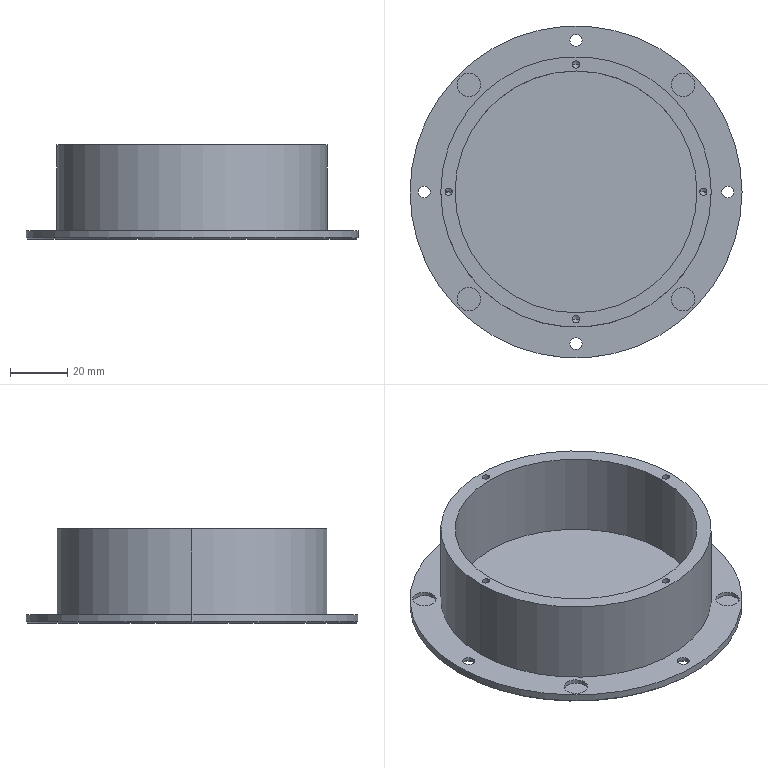Part | SolidWorks | features HoleWzd 2, ICE 2, Chamfer 1, Extrusion 1 | 1 solid | 56 faces | box 116 x 116 x 33 mm | volume 73097 mm3 | cylinder 30 | cone 18 | plane 8 | commonest cylinder face diameters 2.5 x8 4.2 x8 8.2 x8 84.5 x2 94.5 x2 116 x2
STEP:
#1=CARTESIAN_POINT('',(-41.577,-37.477,1.6));
#2=VERTEX_POINT('',#1);
#3=CARTESIAN_POINT('',(-33.377,-37.477,1.6));
#4=VERTEX_POINT('',#3);
#5=CARTESIAN_POINT('',(-37.477,-37.477,1.6));
#6=DIRECTION('',(0.,0.,1.));
#7=DIRECTION('',(-1.,0.,0.));
#8=AXIS2_PLACEMENT_3D('',#5,#6,#7);
#9=CIRCLE('',#8,4.1);
#10=EDGE_CURVE('',#2,#4,#9,.T.);
#11=ORIENTED_EDGE('',*,*,#10,.F.);
#12=CARTESIAN_POINT('',(-41.577,-37.477,3.));
#13=VERTEX_POINT('',#12);
#14=CARTESIAN_POINT('',(-41.577,-37.477,1.6));
#15=DIRECTION('',(0.,0.,1.));
#16=VECTOR('',#15,1000.);
#17=LINE('',#14,#16);
#18=EDGE_CURVE('',#2,#13,#17,.T.);
#19=ORIENTED_EDGE('',*,*,#18,.T.);
#20=CARTESIAN_POINT('',(-33.377,-37.477,3.));
#21=VERTEX_POINT('',#20);
#22=CARTESIAN_POINT('',(-37.477,-37.477,3.));
#23=DIRECTION('',(0.,0.,1.));
#24=DIRECTION('',(-1.,0.,0.));
#25=AXIS2_PLACEMENT_3D('',#22,#23,#24);
#26=CIRCLE('',#25,4.1);
#27=EDGE_CURVE('',#13,#21,#26,.T.);
#28=ORIENTED_EDGE('',*,*,#27,.T.);
#29=CARTESIAN_POINT('',(-33.377,-37.477,1.6));
#30=DIRECTION('',(0.,0.,1.));
#31=VECTOR('',#30,1000.);
#32=LINE('',#29,#31);
#33=EDGE_CURVE('',#4,#21,#32,.T.);
#34=ORIENTED_EDGE('',*,*,#33,.F.);
#35=EDGE_LOOP('',(#11,#19,#28,#34));
#36=FACE_OUTER_BOUND('',#35,.T.);
#37=CARTESIAN_POINT('',(-37.477,-37.477,1.6));
#38=DIRECTION('',(0.,0.,1.));
#39=DIRECTION('',(1.,0.,0.));
#40=AXIS2_PLACEMENT_3D('',#37,#38,#39);
#41=CYLINDRICAL_SURFACE('',#40,4.1);
#42=ADVANCED_FACE('',(#36),#41,.F.);
#43=CARTESIAN_POINT('',(-41.577,37.477,1.6));
#44=VERTEX_POINT('',#43);
#45=CARTESIAN_POINT('',(-33.377,37.477,1.6));
#46=VERTEX_POINT('',#45);
#47=CARTESIAN_POINT('',(-37.477,37.477,1.6));
#48=DIRECTION('',(0.,0.,1.));
#49=DIRECTION('',(1.,0.,0.));
#50=AXIS2_PLACEMENT_3D('',#47,#48,#49);
#51=CIRCLE('',#50,4.1);
#52=EDGE_CURVE('',#44,#46,#51,.T.);
#53=ORIENTED_EDGE('',*,*,#52,.F.);
#54=CARTESIAN_POINT('',(-41.577,37.477,3.));
#55=VERTEX_POINT('',#54);
#56=CARTESIAN_POINT('',(-41.577,37.477,1.6));
#57=DIRECTION('',(0.,0.,1.));
#58=VECTOR('',#57,1000.);
#59=LINE('',#56,#58);
#60=EDGE_CURVE('',#44,#55,#59,.T.);
#61=ORIENTED_EDGE('',*,*,#60,.T.);
#62=CARTESIAN_POINT('',(-33.377,37.477,3.));
#63=VERTEX_POINT('',#62);
#64=CARTESIAN_POINT('',(-37.477,37.477,3.));
#65=DIRECTION('',(0.,0.,1.));
#66=DIRECTION('',(1.,0.,0.));
#67=AXIS2_PLACEMENT_3D('',#64,#65,#66);
#68=CIRCLE('',#67,4.1);
#69=EDGE_CURVE('',#55,#63,#68,.T.);
#70=ORIENTED_EDGE('',*,*,#69,.T.);
#71=CARTESIAN_POINT('',(-33.377,37.477,1.6));
#72=DIRECTION('',(0.,0.,1.));
#73=VECTOR('',#72,1000.);
#74=LINE('',#71,#73);
#75=EDGE_CURVE('',#46,#63,#74,.T.);
#76=ORIENTED_EDGE('',*,*,#75,.F.);
#77=EDGE_LOOP('',(#53,#61,#70,#76));
#78=FACE_OUTER_BOUND('',#77,.T.);
#79=CARTESIAN_POINT('',(-37.477,37.477,1.6));
#80=DIRECTION('',(0.,0.,1.));
#81=DIRECTION('',(1.,0.,0.));
#82=AXIS2_PLACEMENT_3D('',#79,#80,#81);
#83=CYLINDRICAL_SURFACE('',#82,4.1);
#84=ADVANCED_FACE('',(#78),#83,.F.);
#85=CARTESIAN_POINT('',(33.377,37.477,1.6));
#86=VERTEX_POINT('',#85);
#87=CARTESIAN_POINT('',(41.577,37.477,1.6));
#88=VERTEX_POINT('',#87);
#89=CARTESIAN_POINT('',(37.477,37.477,1.6));
#90=DIRECTION('',(0.,0.,1.));
#91=DIRECTION('',(-1.,0.,0.));
#92=AXIS2_PLACEMENT_3D('',#89,#90,#91);
#93=CIRCLE('',#92,4.1);
#94=EDGE_CURVE('',#86,#88,#93,.T.);
#95=ORIENTED_EDGE('',*,*,#94,.F.);
#96=CARTESIAN_POINT('',(33.377,37.477,3.));
#97=VERTEX_POINT('',#96);
#98=CARTESIAN_POINT('',(33.377,37.477,1.6));
#99=DIRECTION('',(0.,0.,1.));
#100=VECTOR('',#99,1000.);
#101=LINE('',#98,#100);
#102=EDGE_CURVE('',#86,#97,#101,.T.);
#103=ORIENTED_EDGE('',*,*,#102,.T.);
#104=CARTESIAN_POINT('',(41.577,37.477,3.));
#105=VERTEX_POINT('',#104);
#106=CARTESIAN_POINT('',(37.477,37.477,3.));
#107=DIRECTION('',(0.,0.,1.));
#108=DIRECTION('',(-1.,0.,0.));
#109=AXIS2_PLACEMENT_3D('',#106,#107,#108);
#110=CIRCLE('',#109,4.1);
#111=EDGE_CURVE('',#97,#105,#110,.T.);
#112=ORIENTED_EDGE('',*,*,#111,.T.);
#113=CARTESIAN_POINT('',(41.577,37.477,1.6));
#114=DIRECTION('',(0.,0.,1.));
#115=VECTOR('',#114,1000.);
#116=LINE('',#113,#115);
#117=EDGE_CURVE('',#88,#105,#116,.T.);
#118=ORIENTED_EDGE('',*,*,#117,.F.);
#119=EDGE_LOOP('',(#95,#103,#112,#118));
#120=FACE_OUTER_BOUND('',#119,.T.);
#121=CARTESIAN_POINT('',(37.477,37.477,1.6));
#122=DIRECTION('',(0.,0.,1.));
#123=DIRECTION('',(1.,0.,0.));
#124=AXIS2_PLACEMENT_3D('',#121,#122,#123);
#125=CYLINDRICAL_SURFACE('',#124,4.1);
#126=ADVANCED_FACE('',(#120),#125,.F.);
#127=CARTESIAN_POINT('',(33.377,-37.477,1.6));
#128=VERTEX_POINT('',#127);
#129=CARTESIAN_POINT('',(41.577,-37.477,1.6));
#130=VERTEX_POINT('',#129);
#131=CARTESIAN_POINT('',(37.477,-37.477,1.6));
#132=DIRECTION('',(0.,0.,1.));
#133=DIRECTION('',(1.,0.,0.));
#134=AXIS2_PLACEMENT_3D('',#131,#132,#133);
#135=CIRCLE('',#134,4.1);
#136=EDGE_CURVE('',#128,#130,#135,.T.);
#137=ORIENTED_EDGE('',*,*,#136,.F.);
#138=CARTESIAN_POINT('',(33.377,-37.477,3.));
#139=VERTEX_POINT('',#138);
#140=CARTESIAN_POINT('',(33.377,-37.477,1.6));
#141=DIRECTION('',(0.,0.,1.));
#142=VECTOR('',#141,1000.);
#143=LINE('',#140,#142);
#144=EDGE_CURVE('',#128,#139,#143,.T.);
#145=ORIENTED_EDGE('',*,*,#144,.T.);
#146=CARTESIAN_POINT('',(41.577,-37.477,3.));
#147=VERTEX_POINT('',#146);
#148=CARTESIAN_POINT('',(37.477,-37.477,3.));
#149=DIRECTION('',(0.,0.,1.));
#150=DIRECTION('',(1.,0.,0.));
#151=AXIS2_PLACEMENT_3D('',#148,#149,#150);
#152=CIRCLE('',#151,4.1);
#153=EDGE_CURVE('',#139,#147,#152,.T.);
#154=ORIENTED_EDGE('',*,*,#153,.T.);
#155=CARTESIAN_POINT('',(41.577,-37.477,1.6));
#156=DIRECTION('',(0.,0.,1.));
#157=VECTOR('',#156,1000.);
#158=LINE('',#155,#157);
#159=EDGE_CURVE('',#130,#147,#158,.T.);
#160=ORIENTED_EDGE('',*,*,#159,.F.);
#161=EDGE_LOOP('',(#137,#145,#154,#160));
#162=FACE_OUTER_BOUND('',#161,.T.);
#163=CARTESIAN_POINT('',(37.477,-37.477,1.6));
#164=DIRECTION('',(0.,0.,1.));
#165=DIRECTION('',(1.,0.,0.));
#166=AXIS2_PLACEMENT_3D('',#163,#164,#165);
#167=CYLINDRICAL_SURFACE('',#166,4.1);
#168=ADVANCED_FACE('',(#162),#167,.F.);
#169=CARTESIAN_POINT('',(-1.25,44.5,25.5));
#170=VERTEX_POINT('',#169);
#171=CARTESIAN_POINT('',(1.25,44.5,25.5));
#172=VERTEX_POINT('',#171);
#173=CARTESIAN_POINT('',(0.,44.5,25.5));
#174=DIRECTION('',(0.,0.,1.));
#175=DIRECTION('',(1.,0.,0.));
#176=AXIS2_PLACEMENT_3D('',#173,#174,#175);
#177=CIRCLE('',#176,1.25);
#178=EDGE_CURVE('',#170,#172,#177,.T.);
#179=ORIENTED_EDGE('',*,*,#178,.F.);
#180=CARTESIAN_POINT('',(-1.25,44.5,33.));
#181=VERTEX_POINT('',#180);
#182=CARTESIAN_POINT('',(-1.25,44.5,33.));
#183=DIRECTION('',(0.,0.,1.));
#184=VECTOR('',#183,1000.);
#185=LINE('',#182,#184);
#186=EDGE_CURVE('',#170,#181,#185,.T.);
#187=ORIENTED_EDGE('',*,*,#186,.T.);
#188=CARTESIAN_POINT('',(1.25,44.5,33.));
#189=VERTEX_POINT('',#188);
#190=CARTESIAN_POINT('',(0.,44.5,33.));
#191=DIRECTION('',(0.,0.,1.));
#192=DIRECTION('',(1.,0.,0.));
#193=AXIS2_PLACEMENT_3D('',#190,#191,#192);
#194=CIRCLE('',#193,1.25);
#195=EDGE_CURVE('',#181,#189,#194,.T.);
#196=ORIENTED_EDGE('',*,*,#195,.T.);
#197=CARTESIAN_POINT('',(1.25,44.5,33.));
#198=DIRECTION('',(0.,0.,1.));
#199=VECTOR('',#198,1000.);
#200=LINE('',#197,#199);
#201=EDGE_CURVE('',#172,#189,#200,.T.);
#202=ORIENTED_EDGE('',*,*,#201,.F.);
#203=EDGE_LOOP('',(#179,#187,#196,#202));
#204=FACE_OUTER_BOUND('',#203,.T.);
#205=CARTESIAN_POINT('',(0.,44.5,33.));
#206=DIRECTION('',(0.,0.,1.));
#207=DIRECTION('',(1.,0.,0.));
#208=AXIS2_PLACEMENT_3D('',#205,#206,#207);
#209=CYLINDRICAL_SURFACE('',#208,1.25);
#210=ADVANCED_FACE('',(#204),#209,.F.);
#211=CARTESIAN_POINT('',(0.,44.5,24.749));
#212=VERTEX_POINT('',#211);
#213=CARTESIAN_POINT('',(1.25,44.5,25.5));
#214=DIRECTION('',(0.8572,0.,0.515));
#215=VECTOR('',#214,1000.);
#216=LINE('',#213,#215);
#217=EDGE_CURVE('',#212,#172,#216,.T.);
#218=ORIENTED_EDGE('',*,*,#217,.F.);
#219=CARTESIAN_POINT('',(-1.25,44.5,25.5));
#220=DIRECTION('',(-0.8572,0.,0.515));
#221=VECTOR('',#220,1000.);
#222=LINE('',#219,#221);
#223=EDGE_CURVE('',#212,#170,#222,.T.);
#224=ORIENTED_EDGE('',*,*,#223,.T.);
#225=ORIENTED_EDGE('',*,*,#178,.T.);
#226=EDGE_LOOP('',(#218,#224,#225));
#227=FACE_OUTER_BOUND('',#226,.T.);
#228=CARTESIAN_POINT('',(0.,44.5,25.5));
#229=DIRECTION('',(0.,0.,1.));
#230=DIRECTION('',(1.,0.,0.));
#231=AXIS2_PLACEMENT_3D('',#228,#229,#230);
#232=CONICAL_SURFACE('',#231,1.25,1.03);
#233=ADVANCED_FACE('',(#227),#232,.F.);
#234=CARTESIAN_POINT('',(43.25,0.,25.5));
#235=VERTEX_POINT('',#234);
#236=CARTESIAN_POINT('',(45.75,0.,25.5));
#237=VERTEX_POINT('',#236);
#238=CARTESIAN_POINT('',(44.5,0.,25.5));
#239=DIRECTION('',(0.,0.,1.));
#240=DIRECTION('',(1.,0.,0.));
#241=AXIS2_PLACEMENT_3D('',#238,#239,#240);
#242=CIRCLE('',#241,1.25);
#243=EDGE_CURVE('',#235,#237,#242,.T.);
#244=ORIENTED_EDGE('',*,*,#243,.F.);
#245=CARTESIAN_POINT('',(43.25,0.,33.));
#246=VERTEX_POINT('',#245);
#247=CARTESIAN_POINT('',(43.25,0.,33.));
#248=DIRECTION('',(0.,0.,1.));
#249=VECTOR('',#248,1000.);
#250=LINE('',#247,#249);
#251=EDGE_CURVE('',#235,#246,#250,.T.);
#252=ORIENTED_EDGE('',*,*,#251,.T.);
#253=CARTESIAN_POINT('',(45.75,0.,33.));
#254=VERTEX_POINT('',#253);
#255=CARTESIAN_POINT('',(44.5,0.,33.));
#256=DIRECTION('',(0.,0.,1.));
#257=DIRECTION('',(1.,0.,0.));
#258=AXIS2_PLACEMENT_3D('',#255,#256,#257);
#259=CIRCLE('',#258,1.25);
#260=EDGE_CURVE('',#246,#254,#259,.T.);
#261=ORIENTED_EDGE('',*,*,#260,.T.);
#262=CARTESIAN_POINT('',(45.75,0.,33.));
#263=DIRECTION('',(0.,0.,1.));
#264=VECTOR('',#263,1000.);
#265=LINE('',#262,#264);
#266=EDGE_CURVE('',#237,#254,#265,.T.);
#267=ORIENTED_EDGE('',*,*,#266,.F.);
#268=EDGE_LOOP('',(#244,#252,#261,#267));
#269=FACE_OUTER_BOUND('',#268,.T.);
#270=CARTESIAN_POINT('',(44.5,0.,33.));
#271=DIRECTION('',(0.,0.,1.));
#272=DIRECTION('',(1.,0.,0.));
#273=AXIS2_PLACEMENT_3D('',#270,#271,#272);
#274=CYLINDRICAL_SURFACE('',#273,1.25);
#275=ADVANCED_FACE('',(#269),#274,.F.);
#276=CARTESIAN_POINT('',(44.5,0.,24.749));
#277=VERTEX_POINT('',#276);
#278=CARTESIAN_POINT('',(45.75,0.,25.5));
#279=DIRECTION('',(0.8572,0.,0.515));
#280=VECTOR('',#279,1000.);
#281=LINE('',#278,#280);
#282=EDGE_CURVE('',#277,#237,#281,.T.);
#283=ORIENTED_EDGE('',*,*,#282,.F.);
#284=CARTESIAN_POINT('',(43.25,0.,25.5));
#285=DIRECTION('',(-0.8572,0.,0.515));
#286=VECTOR('',#285,1000.);
#287=LINE('',#284,#286);
#288=EDGE_CURVE('',#277,#235,#287,.T.);
#289=ORIENTED_EDGE('',*,*,#288,.T.);
#290=ORIENTED_EDGE('',*,*,#243,.T.);
#291=EDGE_LOOP('',(#283,#289,#290));
#292=FACE_OUTER_BOUND('',#291,.T.);
#293=CARTESIAN_POINT('',(44.5,0.,25.5));
#294=DIRECTION('',(0.,0.,1.));
#295=DIRECTION('',(1.,0.,0.));
#296=AXIS2_PLACEMENT_3D('',#293,#294,#295);
#297=CONICAL_SURFACE('',#296,1.25,1.03);
#298=ADVANCED_FACE('',(#292),#297,.F.);
#299=CARTESIAN_POINT('',(-1.25,-44.5,25.5));
#300=VERTEX_POINT('',#299);
#301=CARTESIAN_POINT('',(1.25,-44.5,25.5));
#302=VERTEX_POINT('',#301);
#303=CARTESIAN_POINT('',(0.,-44.5,25.5));
#304=DIRECTION('',(0.,0.,1.));
#305=DIRECTION('',(1.,0.,0.));
#306=AXIS2_PLACEMENT_3D('',#303,#304,#305);
#307=CIRCLE('',#306,1.25);
#308=EDGE_CURVE('',#300,#302,#307,.T.);
#309=ORIENTED_EDGE('',*,*,#308,.F.);
#310=CARTESIAN_POINT('',(-1.25,-44.5,33.));
#311=VERTEX_POINT('',#310);
#312=CARTESIAN_POINT('',(-1.25,-44.5,33.));
#313=DIRECTION('',(0.,0.,1.));
#314=VECTOR('',#313,1000.);
#315=LINE('',#312,#314);
#316=EDGE_CURVE('',#300,#311,#315,.T.);
#317=ORIENTED_EDGE('',*,*,#316,.T.);
#318=CARTESIAN_POINT('',(1.25,-44.5,33.));
#319=VERTEX_POINT('',#318);
#320=CARTESIAN_POINT('',(0.,-44.5,33.));
#321=DIRECTION('',(0.,0.,1.));
#322=DIRECTION('',(1.,0.,0.));
#323=AXIS2_PLACEMENT_3D('',#320,#321,#322);
#324=CIRCLE('',#323,1.25);
#325=EDGE_CURVE('',#311,#319,#324,.T.);
#326=ORIENTED_EDGE('',*,*,#325,.T.);
#327=CARTESIAN_POINT('',(1.25,-44.5,33.));
#328=DIRECTION('',(0.,0.,1.));
#329=VECTOR('',#328,1000.);
#330=LINE('',#327,#329);
#331=EDGE_CURVE('',#302,#319,#330,.T.);
#332=ORIENTED_EDGE('',*,*,#331,.F.);
#333=EDGE_LOOP('',(#309,#317,#326,#332));
#334=FACE_OUTER_BOUND('',#333,.T.);
#335=CARTESIAN_POINT('',(0.,-44.5,33.));
#336=DIRECTION('',(0.,0.,1.));
#337=DIRECTION('',(1.,0.,0.));
#338=AXIS2_PLACEMENT_3D('',#335,#336,#337);
#339=CYLINDRICAL_SURFACE('',#338,1.25);
#340=ADVANCED_FACE('',(#334),#339,.F.);
#341=CARTESIAN_POINT('',(0.,-44.5,24.749));
#342=VERTEX_POINT('',#341);
#343=CARTESIAN_POINT('',(1.25,-44.5,25.5));
#344=DIRECTION('',(0.8572,0.,0.515));
#345=VECTOR('',#344,1000.);
#346=LINE('',#343,#345);
#347=EDGE_CURVE('',#342,#302,#346,.T.);
#348=ORIENTED_EDGE('',*,*,#347,.F.);
#349=CARTESIAN_POINT('',(-1.25,-44.5,25.5));
#350=DIRECTION('',(-0.8572,0.,0.515));
#351=VECTOR('',#350,1000.);
#352=LINE('',#349,#351);
#353=EDGE_CURVE('',#342,#300,#352,.T.);
#354=ORIENTED_EDGE('',*,*,#353,.T.);
#355=ORIENTED_EDGE('',*,*,#308,.T.);
#356=EDGE_LOOP('',(#348,#354,#355));
#357=FACE_OUTER_BOUND('',#356,.T.);
#358=CARTESIAN_POINT('',(0.,-44.5,25.5));
#359=DIRECTION('',(0.,0.,1.));
#360=DIRECTION('',(1.,0.,0.));
#361=AXIS2_PLACEMENT_3D('',#358,#359,#360);
#362=CONICAL_SURFACE('',#361,1.25,1.03);
#363=ADVANCED_FACE('',(#357),#362,.F.);
#364=CARTESIAN_POINT('',(-45.75,0.,25.5));
#365=VERTEX_POINT('',#364);
#366=CARTESIAN_POINT('',(-43.25,0.,25.5));
#367=VERTEX_POINT('',#366);
#368=CARTESIAN_POINT('',(-44.5,0.,25.5));
#369=DIRECTION('',(0.,0.,1.));
#370=DIRECTION('',(1.,0.,0.));
#371=AXIS2_PLACEMENT_3D('',#368,#369,#370);
#372=CIRCLE('',#371,1.25);
#373=EDGE_CURVE('',#365,#367,#372,.T.);
#374=ORIENTED_EDGE('',*,*,#373,.F.);
#375=CARTESIAN_POINT('',(-45.75,0.,33.));
#376=VERTEX_POINT('',#375);
#377=CARTESIAN_POINT('',(-45.75,0.,33.));
#378=DIRECTION('',(0.,0.,1.));
#379=VECTOR('',#378,1000.);
#380=LINE('',#377,#379);
#381=EDGE_CURVE('',#365,#376,#380,.T.);
#382=ORIENTED_EDGE('',*,*,#381,.T.);
#383=CARTESIAN_POINT('',(-43.25,0.,33.));
#384=VERTEX_POINT('',#383);
#385=CARTESIAN_POINT('',(-44.5,0.,33.));
#386=DIRECTION('',(0.,0.,1.));
#387=DIRECTION('',(1.,0.,0.));
#388=AXIS2_PLACEMENT_3D('',#385,#386,#387);
#389=CIRCLE('',#388,1.25);
#390=EDGE_CURVE('',#376,#384,#389,.T.);
#391=ORIENTED_EDGE('',*,*,#390,.T.);
#392=CARTESIAN_POINT('',(-43.25,0.,33.));
#393=DIRECTION('',(0.,0.,1.));
#394=VECTOR('',#393,1000.);
#395=LINE('',#392,#394);
#396=EDGE_CURVE('',#367,#384,#395,.T.);
#397=ORIENTED_EDGE('',*,*,#396,.F.);
#398=EDGE_LOOP('',(#374,#382,#391,#397));
#399=FACE_OUTER_BOUND('',#398,.T.);
#400=CARTESIAN_POINT('',(-44.5,0.,33.));
#401=DIRECTION('',(0.,0.,1.));
#402=DIRECTION('',(1.,0.,0.));
#403=AXIS2_PLACEMENT_3D('',#400,#401,#402);
#404=CYLINDRICAL_SURFACE('',#403,1.25);
#405=ADVANCED_FACE('',(#399),#404,.F.);
#406=CARTESIAN_POINT('',(-44.5,0.,24.749));
#407=VERTEX_POINT('',#406);
#408=CARTESIAN_POINT('',(-43.25,0.,25.5));
#409=DIRECTION('',(0.8572,0.,0.515));
#410=VECTOR('',#409,1000.);
#411=LINE('',#408,#410);
#412=EDGE_CURVE('',#407,#367,#411,.T.);
#413=ORIENTED_EDGE('',*,*,#412,.F.);
#414=CARTESIAN_POINT('',(-45.75,0.,25.5));
#415=DIRECTION('',(-0.8572,0.,0.515));
#416=VECTOR('',#415,1000.);
#417=LINE('',#414,#416);
#418=EDGE_CURVE('',#407,#365,#417,.T.);
#419=ORIENTED_EDGE('',*,*,#418,.T.);
#420=ORIENTED_EDGE('',*,*,#373,.T.);
#421=EDGE_LOOP('',(#413,#419,#420));
#422=FACE_OUTER_BOUND('',#421,.T.);
#423=CARTESIAN_POINT('',(-44.5,0.,25.5));
#424=DIRECTION('',(0.,0.,1.));
#425=DIRECTION('',(1.,0.,0.));
#426=AXIS2_PLACEMENT_3D('',#423,#424,#425);
#427=CONICAL_SURFACE('',#426,1.25,1.03);
#428=ADVANCED_FACE('',(#422),#427,.F.);
#429=CARTESIAN_POINT('',(2.1,53.,1.9));
#430=VERTEX_POINT('',#429);
#431=CARTESIAN_POINT('',(-2.1,53.,1.9));
#432=VERTEX_POINT('',#431);
#433=CARTESIAN_POINT('',(0.,53.,1.9));
#434=DIRECTION('',(0.,0.,-1.));
#435=DIRECTION('',(-1.,0.,0.));
#436=AXIS2_PLACEMENT_3D('',#433,#434,#435);
#437=CIRCLE('',#436,2.1);
#438=EDGE_CURVE('',#430,#432,#437,.T.);
#439=ORIENTED_EDGE('',*,*,#438,.F.);
#440=CARTESIAN_POINT('',(4.,53.,0.));
#441=VERTEX_POINT('',#440);
#442=CARTESIAN_POINT('',(4.,53.,0.));
#443=DIRECTION('',(0.7071,0.,-0.7071));
#444=VECTOR('',#443,1000.);
#445=LINE('',#442,#444);
#446=EDGE_CURVE('',#430,#441,#445,.T.);
#447=ORIENTED_EDGE('',*,*,#446,.T.);
#448=CARTESIAN_POINT('',(-4.,53.,0.));
#449=VERTEX_POINT('',#448);
#450=CARTESIAN_POINT('',(0.,53.,0.));
#451=DIRECTION('',(0.,0.,-1.));
#452=DIRECTION('',(-1.,0.,0.));
#453=AXIS2_PLACEMENT_3D('',#450,#451,#452);
#454=CIRCLE('',#453,4.);
#455=EDGE_CURVE('',#441,#449,#454,.T.);
#456=ORIENTED_EDGE('',*,*,#455,.T.);
#457=CARTESIAN_POINT('',(-4.,53.,0.));
#458=DIRECTION('',(-0.7071,0.,-0.7071));
#459=VECTOR('',#458,1000.);
#460=LINE('',#457,#459);
#461=EDGE_CURVE('',#432,#449,#460,.T.);
#462=ORIENTED_EDGE('',*,*,#461,.F.);
#463=EDGE_LOOP('',(#439,#447,#456,#462));
#464=FACE_OUTER_BOUND('',#463,.T.);
#465=CARTESIAN_POINT('',(0.,53.,0.));
#466=DIRECTION('',(0.,0.,-1.));
#467=DIRECTION('',(-1.,0.,0.));
#468=AXIS2_PLACEMENT_3D('',#465,#466,#467);
#469=CONICAL_SURFACE('',#468,4.,0.7854);
#470=ADVANCED_FACE('',(#464),#469,.F.);
#471=CARTESIAN_POINT('',(-2.1,53.,3.));
#472=VERTEX_POINT('',#471);
#473=CARTESIAN_POINT('',(2.1,53.,3.));
#474=VERTEX_POINT('',#473);
#475=CARTESIAN_POINT('',(0.,53.,3.));
#476=DIRECTION('',(0.,0.,1.));
#477=DIRECTION('',(1.,0.,0.));
#478=AXIS2_PLACEMENT_3D('',#475,#476,#477);
#479=CIRCLE('',#478,2.1);
#480=EDGE_CURVE('',#472,#474,#479,.T.);
#481=ORIENTED_EDGE('',*,*,#480,.T.);
#482=CARTESIAN_POINT('',(2.1,53.,0.));
#483=DIRECTION('',(0.,0.,-1.));
#484=VECTOR('',#483,1000.);
#485=LINE('',#482,#484);
#486=EDGE_CURVE('',#474,#430,#485,.T.);
#487=ORIENTED_EDGE('',*,*,#486,.T.);
#488=ORIENTED_EDGE('',*,*,#438,.T.);
#489=CARTESIAN_POINT('',(-2.1,53.,0.));
#490=DIRECTION('',(0.,0.,-1.));
#491=VECTOR('',#490,1000.);
#492=LINE('',#489,#491);
#493=EDGE_CURVE('',#472,#432,#492,.T.);
#494=ORIENTED_EDGE('',*,*,#493,.F.);
#495=EDGE_LOOP('',(#481,#487,#488,#494));
#496=FACE_OUTER_BOUND('',#495,.T.);
#497=CARTESIAN_POINT('',(0.,53.,0.));
#498=DIRECTION('',(0.,0.,-1.));
#499=DIRECTION('',(-1.,0.,0.));
#500=AXIS2_PLACEMENT_3D('',#497,#498,#499);
#501=CYLINDRICAL_SURFACE('',#500,2.1);
#502=ADVANCED_FACE('',(#496),#501,.F.);
#503=CARTESIAN_POINT('',(-50.9,0.,1.9));
#504=VERTEX_POINT('',#503);
#505=CARTESIAN_POINT('',(-55.1,0.,1.9));
#506=VERTEX_POINT('',#505);
#507=CARTESIAN_POINT('',(-53.,0.,1.9));
#508=DIRECTION('',(0.,0.,-1.));
#509=DIRECTION('',(-1.,0.,0.));
#510=AXIS2_PLACEMENT_3D('',#507,#508,#509);
#511=CIRCLE('',#510,2.1);
#512=EDGE_CURVE('',#504,#506,#511,.T.);
#513=ORIENTED_EDGE('',*,*,#512,.F.);
#514=CARTESIAN_POINT('',(-49.,0.,0.));
#515=VERTEX_POINT('',#514);
#516=CARTESIAN_POINT('',(-49.,0.,0.));
#517=DIRECTION('',(0.7071,0.,-0.7071));
#518=VECTOR('',#517,1000.);
#519=LINE('',#516,#518);
#520=EDGE_CURVE('',#504,#515,#519,.T.);
#521=ORIENTED_EDGE('',*,*,#520,.T.);
#522=CARTESIAN_POINT('',(-57.,0.,0.));
#523=VERTEX_POINT('',#522);
#524=CARTESIAN_POINT('',(-53.,0.,0.));
#525=DIRECTION('',(0.,0.,-1.));
#526=DIRECTION('',(-1.,0.,0.));
#527=AXIS2_PLACEMENT_3D('',#524,#525,#526);
#528=CIRCLE('',#527,4.);
#529=EDGE_CURVE('',#515,#523,#528,.T.);
#530=ORIENTED_EDGE('',*,*,#529,.T.);
#531=CARTESIAN_POINT('',(-57.,0.,0.));
#532=DIRECTION('',(-0.7071,0.,-0.7071));
#533=VECTOR('',#532,1000.);
#534=LINE('',#531,#533);
#535=EDGE_CURVE('',#506,#523,#534,.T.);
#536=ORIENTED_EDGE('',*,*,#535,.F.);
#537=EDGE_LOOP('',(#513,#521,#530,#536));
#538=FACE_OUTER_BOUND('',#537,.T.);
#539=CARTESIAN_POINT('',(-53.,0.,0.));
#540=DIRECTION('',(0.,0.,-1.));
#541=DIRECTION('',(-1.,0.,0.));
#542=AXIS2_PLACEMENT_3D('',#539,#540,#541);
#543=CONICAL_SURFACE('',#542,4.,0.7854);
#544=ADVANCED_FACE('',(#538),#543,.F.);
#545=CARTESIAN_POINT('',(-55.1,0.,3.));
#546=VERTEX_POINT('',#545);
#547=CARTESIAN_POINT('',(-50.9,0.,3.));
#548=VERTEX_POINT('',#547);
#549=CARTESIAN_POINT('',(-53.,0.,3.));
#550=DIRECTION('',(0.,0.,1.));
#551=DIRECTION('',(1.,0.,0.));
#552=AXIS2_PLACEMENT_3D('',#549,#550,#551);
#553=CIRCLE('',#552,2.1);
#554=EDGE_CURVE('',#546,#548,#553,.T.);
#555=ORIENTED_EDGE('',*,*,#554,.T.);
#556=CARTESIAN_POINT('',(-50.9,0.,0.));
#557=DIRECTION('',(0.,0.,-1.));
#558=VECTOR('',#557,1000.);
#559=LINE('',#556,#558);
#560=EDGE_CURVE('',#548,#504,#559,.T.);
#561=ORIENTED_EDGE('',*,*,#560,.T.);
#562=ORIENTED_EDGE('',*,*,#512,.T.);
#563=CARTESIAN_POINT('',(-55.1,0.,0.));
#564=DIRECTION('',(0.,0.,-1.));
#565=VECTOR('',#564,1000.);
#566=LINE('',#563,#565);
#567=EDGE_CURVE('',#546,#506,#566,.T.);
#568=ORIENTED_EDGE('',*,*,#567,.F.);
#569=EDGE_LOOP('',(#555,#561,#562,#568));
#570=FACE_OUTER_BOUND('',#569,.T.);
#571=CARTESIAN_POINT('',(-53.,0.,0.));
#572=DIRECTION('',(0.,0.,-1.));
#573=DIRECTION('',(-1.,0.,0.));
#574=AXIS2_PLACEMENT_3D('',#571,#572,#573);
#575=CYLINDRICAL_SURFACE('',#574,2.1);
#576=ADVANCED_FACE('',(#570),#575,.F.);
#577=CARTESIAN_POINT('',(2.1,-53.,1.9));
#578=VERTEX_POINT('',#577);
#579=CARTESIAN_POINT('',(-2.1,-53.,1.9));
#580=VERTEX_POINT('',#579);
#581=CARTESIAN_POINT('',(0.,-53.,1.9));
#582=DIRECTION('',(0.,0.,-1.));
#583=DIRECTION('',(-1.,0.,0.));
#584=AXIS2_PLACEMENT_3D('',#581,#582,#583);
#585=CIRCLE('',#584,2.1);
#586=EDGE_CURVE('',#578,#580,#585,.T.);
#587=ORIENTED_EDGE('',*,*,#586,.F.);
#588=CARTESIAN_POINT('',(4.,-53.,0.));
#589=VERTEX_POINT('',#588);
#590=CARTESIAN_POINT('',(4.,-53.,0.));
#591=DIRECTION('',(0.7071,0.,-0.7071));
#592=VECTOR('',#591,1000.);
#593=LINE('',#590,#592);
#594=EDGE_CURVE('',#578,#589,#593,.T.);
#595=ORIENTED_EDGE('',*,*,#594,.T.);
#596=CARTESIAN_POINT('',(-4.,-53.,0.));
#597=VERTEX_POINT('',#596);
#598=CARTESIAN_POINT('',(0.,-53.,0.));
#599=DIRECTION('',(0.,0.,-1.));
#600=DIRECTION('',(-1.,0.,0.));
#601=AXIS2_PLACEMENT_3D('',#598,#599,#600);
#602=CIRCLE('',#601,4.);
#603=EDGE_CURVE('',#589,#597,#602,.T.);
#604=ORIENTED_EDGE('',*,*,#603,.T.);
#605=CARTESIAN_POINT('',(-4.,-53.,0.));
#606=DIRECTION('',(-0.7071,0.,-0.7071));
#607=VECTOR('',#606,1000.);
#608=LINE('',#605,#607);
#609=EDGE_CURVE('',#580,#597,#608,.T.);
#610=ORIENTED_EDGE('',*,*,#609,.F.);
#611=EDGE_LOOP('',(#587,#595,#604,#610));
#612=FACE_OUTER_BOUND('',#611,.T.);
#613=CARTESIAN_POINT('',(0.,-53.,0.));
#614=DIRECTION('',(0.,0.,-1.));
#615=DIRECTION('',(-1.,0.,0.));
#616=AXIS2_PLACEMENT_3D('',#613,#614,#615);
#617=CONICAL_SURFACE('',#616,4.,0.7854);
#618=ADVANCED_FACE('',(#612),#617,.F.);
#619=CARTESIAN_POINT('',(-2.1,-53.,3.));
#620=VERTEX_POINT('',#619);
#621=CARTESIAN_POINT('',(2.1,-53.,3.));
#622=VERTEX_POINT('',#621);
#623=CARTESIAN_POINT('',(0.,-53.,3.));
#624=DIRECTION('',(0.,0.,1.));
#625=DIRECTION('',(1.,0.,0.));
#626=AXIS2_PLACEMENT_3D('',#623,#624,#625);
#627=CIRCLE('',#626,2.1);
#628=EDGE_CURVE('',#620,#622,#627,.T.);
#629=ORIENTED_EDGE('',*,*,#628,.T.);
#630=CARTESIAN_POINT('',(2.1,-53.,0.));
#631=DIRECTION('',(0.,0.,-1.));
#632=VECTOR('',#631,1000.);
#633=LINE('',#630,#632);
#634=EDGE_CURVE('',#622,#578,#633,.T.);
#635=ORIENTED_EDGE('',*,*,#634,.T.);
#636=ORIENTED_EDGE('',*,*,#586,.T.);
#637=CARTESIAN_POINT('',(-2.1,-53.,0.));
#638=DIRECTION('',(0.,0.,-1.));
#639=VECTOR('',#638,1000.);
#640=LINE('',#637,#639);
#641=EDGE_CURVE('',#620,#580,#640,.T.);
#642=ORIENTED_EDGE('',*,*,#641,.F.);
#643=EDGE_LOOP('',(#629,#635,#636,#642));
#644=FACE_OUTER_BOUND('',#643,.T.);
#645=CARTESIAN_POINT('',(0.,-53.,0.));
#646=DIRECTION('',(0.,0.,-1.));
#647=DIRECTION('',(-1.,0.,0.));
#648=AXIS2_PLACEMENT_3D('',#645,#646,#647);
#649=CYLINDRICAL_SURFACE('',#648,2.1);
#650=ADVANCED_FACE('',(#644),#649,.F.);
#651=CARTESIAN_POINT('',(55.1,0.,1.9));
#652=VERTEX_POINT('',#651);
#653=CARTESIAN_POINT('',(50.9,0.,1.9));
#654=VERTEX_POINT('',#653);
#655=CARTESIAN_POINT('',(53.,0.,1.9));
#656=DIRECTION('',(0.,0.,-1.));
#657=DIRECTION('',(-1.,0.,0.));
#658=AXIS2_PLACEMENT_3D('',#655,#656,#657);
#659=CIRCLE('',#658,2.1);
#660=EDGE_CURVE('',#652,#654,#659,.T.);
#661=ORIENTED_EDGE('',*,*,#660,.F.);
#662=CARTESIAN_POINT('',(57.,0.,0.));
#663=VERTEX_POINT('',#662);
#664=CARTESIAN_POINT('',(57.,0.,0.));
#665=DIRECTION('',(0.7071,0.,-0.7071));
#666=VECTOR('',#665,1000.);
#667=LINE('',#664,#666);
#668=EDGE_CURVE('',#652,#663,#667,.T.);
#669=ORIENTED_EDGE('',*,*,#668,.T.);
#670=CARTESIAN_POINT('',(49.,0.,0.));
#671=VERTEX_POINT('',#670);
#672=CARTESIAN_POINT('',(53.,0.,0.));
#673=DIRECTION('',(0.,0.,-1.));
#674=DIRECTION('',(-1.,0.,0.));
#675=AXIS2_PLACEMENT_3D('',#672,#673,#674);
#676=CIRCLE('',#675,4.);
#677=EDGE_CURVE('',#663,#671,#676,.T.);
#678=ORIENTED_EDGE('',*,*,#677,.T.);
#679=CARTESIAN_POINT('',(49.,0.,0.));
#680=DIRECTION('',(-0.7071,0.,-0.7071));
#681=VECTOR('',#680,1000.);
#682=LINE('',#679,#681);
#683=EDGE_CURVE('',#654,#671,#682,.T.);
#684=ORIENTED_EDGE('',*,*,#683,.F.);
#685=EDGE_LOOP('',(#661,#669,#678,#684));
#686=FACE_OUTER_BOUND('',#685,.T.);
#687=CARTESIAN_POINT('',(53.,0.,0.));
#688=DIRECTION('',(0.,0.,-1.));
#689=DIRECTION('',(-1.,0.,0.));
#690=AXIS2_PLACEMENT_3D('',#687,#688,#689);
#691=CONICAL_SURFACE('',#690,4.,0.7854);
#692=ADVANCED_FACE('',(#686),#691,.F.);
#693=CARTESIAN_POINT('',(50.9,0.,3.));
#694=VERTEX_POINT('',#693);
#695=CARTESIAN_POINT('',(55.1,0.,3.));
#696=VERTEX_POINT('',#695);
#697=CARTESIAN_POINT('',(53.,0.,3.));
#698=DIRECTION('',(0.,0.,1.));
#699=DIRECTION('',(1.,0.,0.));
#700=AXIS2_PLACEMENT_3D('',#697,#698,#699);
#701=CIRCLE('',#700,2.1);
#702=EDGE_CURVE('',#694,#696,#701,.T.);
#703=ORIENTED_EDGE('',*,*,#702,.T.);
#704=CARTESIAN_POINT('',(55.1,0.,0.));
#705=DIRECTION('',(0.,0.,-1.));
#706=VECTOR('',#705,1000.);
#707=LINE('',#704,#706);
#708=EDGE_CURVE('',#696,#652,#707,.T.);
#709=ORIENTED_EDGE('',*,*,#708,.T.);
#710=ORIENTED_EDGE('',*,*,#660,.T.);
#711=CARTESIAN_POINT('',(50.9,0.,0.));
#712=DIRECTION('',(0.,0.,-1.));
#713=VECTOR('',#712,1000.);
#714=LINE('',#711,#713);
#715=EDGE_CURVE('',#694,#654,#714,.T.);
#716=ORIENTED_EDGE('',*,*,#715,.F.);
#717=EDGE_LOOP('',(#703,#709,#710,#716));
#718=FACE_OUTER_BOUND('',#717,.T.);
#719=CARTESIAN_POINT('',(53.,0.,0.));
#720=DIRECTION('',(0.,0.,-1.));
#721=DIRECTION('',(-1.,0.,0.));
#722=AXIS2_PLACEMENT_3D('',#719,#720,#721);
#723=CYLINDRICAL_SURFACE('',#722,2.1);
#724=ADVANCED_FACE('',(#718),#723,.F.);
#725=CARTESIAN_POINT('',(-57.5,0.,0.));
#726=VERTEX_POINT('',#725);
#727=CARTESIAN_POINT('',(57.5,0.,0.));
#728=VERTEX_POINT('',#727);
#729=CARTESIAN_POINT('',(0.,0.,0.));
#730=DIRECTION('',(0.,0.,-1.));
#731=DIRECTION('',(1.,0.,0.));
#732=AXIS2_PLACEMENT_3D('',#729,#730,#731);
#733=CIRCLE('',#732,57.5);
#734=EDGE_CURVE('',#726,#728,#733,.T.);
#735=ORIENTED_EDGE('',*,*,#734,.F.);
#736=CARTESIAN_POINT('',(-58.,0.,0.5));
#737=VERTEX_POINT('',#736);
#738=CARTESIAN_POINT('',(-58.,0.,0.5));
#739=DIRECTION('',(-0.7071,0.,0.7071));
#740=VECTOR('',#739,1000.);
#741=LINE('',#738,#740);
#742=EDGE_CURVE('',#726,#737,#741,.T.);
#743=ORIENTED_EDGE('',*,*,#742,.T.);
#744=CARTESIAN_POINT('',(58.,0.,0.5));
#745=VERTEX_POINT('',#744);
#746=CARTESIAN_POINT('',(0.,0.,0.5));
#747=DIRECTION('',(0.,0.,1.));
#748=DIRECTION('',(1.,0.,0.));
#749=AXIS2_PLACEMENT_3D('',#746,#747,#748);
#750=CIRCLE('',#749,58.);
#751=EDGE_CURVE('',#745,#737,#750,.T.);
#752=ORIENTED_EDGE('',*,*,#751,.F.);
#753=CARTESIAN_POINT('',(58.,0.,0.5));
#754=DIRECTION('',(0.7071,0.,0.7071));
#755=VECTOR('',#754,1000.);
#756=LINE('',#753,#755);
#757=EDGE_CURVE('',#728,#745,#756,.T.);
#758=ORIENTED_EDGE('',*,*,#757,.F.);
#759=EDGE_LOOP('',(#735,#743,#752,#758));
#760=FACE_OUTER_BOUND('',#759,.T.);
#761=CARTESIAN_POINT('',(0.,0.,0.5));
#762=DIRECTION('',(0.,0.,1.));
#763=DIRECTION('',(1.,0.,0.));
#764=AXIS2_PLACEMENT_3D('',#761,#762,#763);
#765=CONICAL_SURFACE('',#764,58.,0.7854);
#766=ADVANCED_FACE('',(#760),#765,.T.);
#767=CARTESIAN_POINT('',(-42.25,0.,33.));
#768=VERTEX_POINT('',#767);
#769=CARTESIAN_POINT('',(42.25,0.,33.));
#770=VERTEX_POINT('',#769);
#771=CARTESIAN_POINT('',(0.,0.,33.));
#772=DIRECTION('',(0.,0.,1.));
#773=DIRECTION('',(1.,0.,0.));
#774=AXIS2_PLACEMENT_3D('',#771,#772,#773);
#775=CIRCLE('',#774,42.25);
#776=EDGE_CURVE('',#768,#770,#775,.T.);
#777=ORIENTED_EDGE('',*,*,#776,.T.);
#778=CARTESIAN_POINT('',(42.25,0.,3.));
#779=VERTEX_POINT('',#778);
#780=CARTESIAN_POINT('',(42.25,0.,33.));
#781=DIRECTION('',(0.,0.,-1.));
#782=VECTOR('',#781,1000.);
#783=LINE('',#780,#782);
#784=EDGE_CURVE('',#770,#779,#783,.T.);
#785=ORIENTED_EDGE('',*,*,#784,.T.);
#786=CARTESIAN_POINT('',(-42.25,0.,3.));
#787=VERTEX_POINT('',#786);
#788=CARTESIAN_POINT('',(0.,0.,3.));
#789=DIRECTION('',(0.,0.,-1.));
#790=DIRECTION('',(1.,0.,0.));
#791=AXIS2_PLACEMENT_3D('',#788,#789,#790);
#792=CIRCLE('',#791,42.25);
#793=EDGE_CURVE('',#779,#787,#792,.T.);
#794=ORIENTED_EDGE('',*,*,#793,.T.);
#795=CARTESIAN_POINT('',(-42.25,0.,33.));
#796=DIRECTION('',(0.,0.,-1.));
#797=VECTOR('',#796,1000.);
#798=LINE('',#795,#797);
#799=EDGE_CURVE('',#768,#787,#798,.T.);
#800=ORIENTED_EDGE('',*,*,#799,.F.);
#801=EDGE_LOOP('',(#777,#785,#794,#800));
#802=FACE_OUTER_BOUND('',#801,.T.);
#803=CARTESIAN_POINT('',(0.,0.,33.));
#804=DIRECTION('',(0.,0.,-1.));
#805=DIRECTION('',(-1.,0.,0.));
#806=AXIS2_PLACEMENT_3D('',#803,#804,#805);
#807=CYLINDRICAL_SURFACE('',#806,42.25);
#808=ADVANCED_FACE('',(#802),#807,.F.);
#809=CARTESIAN_POINT('',(47.25,0.,33.));
#810=VERTEX_POINT('',#809);
#811=CARTESIAN_POINT('',(-47.25,0.,33.));
#812=VERTEX_POINT('',#811);
#813=CARTESIAN_POINT('',(0.,0.,33.));
#814=DIRECTION('',(0.,0.,1.));
#815=DIRECTION('',(1.,0.,0.));
#816=AXIS2_PLACEMENT_3D('',#813,#814,#815);
#817=CIRCLE('',#816,47.25);
#818=EDGE_CURVE('',#810,#812,#817,.T.);
#819=ORIENTED_EDGE('',*,*,#818,.F.);
#820=CARTESIAN_POINT('',(47.25,0.,3.));
#821=VERTEX_POINT('',#820);
#822=CARTESIAN_POINT('',(47.25,0.,33.));
#823=DIRECTION('',(0.,0.,-1.));
#824=VECTOR('',#823,1000.);
#825=LINE('',#822,#824);
#826=EDGE_CURVE('',#810,#821,#825,.T.);
#827=ORIENTED_EDGE('',*,*,#826,.T.);
#828=CARTESIAN_POINT('',(-47.25,0.,3.));
#829=VERTEX_POINT('',#828);
#830=CARTESIAN_POINT('',(0.,0.,3.));
#831=DIRECTION('',(0.,0.,1.));
#832=DIRECTION('',(1.,0.,0.));
#833=AXIS2_PLACEMENT_3D('',#830,#831,#832);
#834=CIRCLE('',#833,47.25);
#835=EDGE_CURVE('',#821,#829,#834,.T.);
#836=ORIENTED_EDGE('',*,*,#835,.T.);
#837=CARTESIAN_POINT('',(-47.25,0.,33.));
#838=DIRECTION('',(0.,0.,-1.));
#839=VECTOR('',#838,1000.);
#840=LINE('',#837,#839);
#841=EDGE_CURVE('',#812,#829,#840,.T.);
#842=ORIENTED_EDGE('',*,*,#841,.F.);
#843=EDGE_LOOP('',(#819,#827,#836,#842));
#844=FACE_OUTER_BOUND('',#843,.T.);
#845=CARTESIAN_POINT('',(0.,0.,33.));
#846=DIRECTION('',(0.,0.,-1.));
#847=DIRECTION('',(-1.,0.,0.));
#848=AXIS2_PLACEMENT_3D('',#845,#846,#847);
#849=CYLINDRICAL_SURFACE('',#848,47.25);
#850=ADVANCED_FACE('',(#844),#849,.T.);
#851=CARTESIAN_POINT('',(58.,0.,3.));
#852=VERTEX_POINT('',#851);
#853=CARTESIAN_POINT('',(-58.,0.,3.));
#854=VERTEX_POINT('',#853);
#855=CARTESIAN_POINT('',(0.,0.,3.));
#856=DIRECTION('',(0.,0.,1.));
#857=DIRECTION('',(1.,0.,0.));
#858=AXIS2_PLACEMENT_3D('',#855,#856,#857);
#859=CIRCLE('',#858,58.);
#860=EDGE_CURVE('',#852,#854,#859,.T.);
#861=ORIENTED_EDGE('',*,*,#860,.F.);
#862=CARTESIAN_POINT('',(58.,0.,3.));
#863=DIRECTION('',(0.,0.,-1.));
#864=VECTOR('',#863,1000.);
#865=LINE('',#862,#864);
#866=EDGE_CURVE('',#852,#745,#865,.T.);
#867=ORIENTED_EDGE('',*,*,#866,.T.);
#868=ORIENTED_EDGE('',*,*,#751,.T.);
#869=CARTESIAN_POINT('',(-58.,0.,3.));
#870=DIRECTION('',(0.,0.,-1.));
#871=VECTOR('',#870,1000.);
#872=LINE('',#869,#871);
#873=EDGE_CURVE('',#854,#737,#872,.T.);
#874=ORIENTED_EDGE('',*,*,#873,.F.);
#875=EDGE_LOOP('',(#861,#867,#868,#874));
#876=FACE_OUTER_BOUND('',#875,.T.);
#877=CARTESIAN_POINT('',(0.,0.,3.));
#878=DIRECTION('',(0.,0.,-1.));
#879=DIRECTION('',(-1.,0.,0.));
#880=AXIS2_PLACEMENT_3D('',#877,#878,#879);
#881=CYLINDRICAL_SURFACE('',#880,58.);
#882=ADVANCED_FACE('',(#876),#881,.T.);
#883=ORIENTED_EDGE('',*,*,#866,.F.);
#884=CARTESIAN_POINT('',(0.,0.,3.));
#885=DIRECTION('',(0.,0.,1.));
#886=DIRECTION('',(1.,0.,0.));
#887=AXIS2_PLACEMENT_3D('',#884,#885,#886);
#888=CIRCLE('',#887,58.);
#889=EDGE_CURVE('',#854,#852,#888,.T.);
#890=ORIENTED_EDGE('',*,*,#889,.F.);
#891=ORIENTED_EDGE('',*,*,#873,.T.);
#892=CARTESIAN_POINT('',(0.,0.,0.5));
#893=DIRECTION('',(0.,0.,1.));
#894=DIRECTION('',(1.,0.,0.));
#895=AXIS2_PLACEMENT_3D('',#892,#893,#894);
#896=CIRCLE('',#895,58.);
#897=EDGE_CURVE('',#737,#745,#896,.T.);
#898=ORIENTED_EDGE('',*,*,#897,.T.);
#899=EDGE_LOOP('',(#883,#890,#891,#898));
#900=FACE_OUTER_BOUND('',#899,.T.);
#901=CARTESIAN_POINT('',(0.,0.,3.));
#902=DIRECTION('',(0.,0.,-1.));
#903=DIRECTION('',(-1.,0.,0.));
#904=AXIS2_PLACEMENT_3D('',#901,#902,#903);
#905=CYLINDRICAL_SURFACE('',#904,58.);
#906=ADVANCED_FACE('',(#900),#905,.T.);
#907=CARTESIAN_POINT('',(-37.477,-37.477,3.));
#908=DIRECTION('',(0.,0.,1.));
#909=DIRECTION('',(-1.,0.,0.));
#910=AXIS2_PLACEMENT_3D('',#907,#908,#909);
#911=CIRCLE('',#910,4.1);
#912=EDGE_CURVE('',#21,#13,#911,.T.);
#913=ORIENTED_EDGE('',*,*,#912,.F.);
#914=ORIENTED_EDGE('',*,*,#27,.F.);
#915=EDGE_LOOP('',(#913,#914));
#916=FACE_BOUND('',#915,.T.);
#917=CARTESIAN_POINT('',(-37.477,37.477,3.));
#918=DIRECTION('',(0.,0.,1.));
#919=DIRECTION('',(1.,0.,0.));
#920=AXIS2_PLACEMENT_3D('',#917,#918,#919);
#921=CIRCLE('',#920,4.1);
#922=EDGE_CURVE('',#63,#55,#921,.T.);
#923=ORIENTED_EDGE('',*,*,#922,.F.);
#924=ORIENTED_EDGE('',*,*,#69,.F.);
#925=EDGE_LOOP('',(#923,#924));
#926=FACE_BOUND('',#925,.T.);
#927=CARTESIAN_POINT('',(37.477,37.477,3.));
#928=DIRECTION('',(0.,0.,1.));
#929=DIRECTION('',(-1.,0.,0.));
#930=AXIS2_PLACEMENT_3D('',#927,#928,#929);
#931=CIRCLE('',#930,4.1);
#932=EDGE_CURVE('',#105,#97,#931,.T.);
#933=ORIENTED_EDGE('',*,*,#932,.F.);
#934=ORIENTED_EDGE('',*,*,#111,.F.);
#935=EDGE_LOOP('',(#933,#934));
#936=FACE_BOUND('',#935,.T.);
#937=CARTESIAN_POINT('',(37.477,-37.477,3.));
#938=DIRECTION('',(0.,0.,1.));
#939=DIRECTION('',(1.,0.,0.));
#940=AXIS2_PLACEMENT_3D('',#937,#938,#939);
#941=CIRCLE('',#940,4.1);
#942=EDGE_CURVE('',#147,#139,#941,.T.);
#943=ORIENTED_EDGE('',*,*,#942,.F.);
#944=ORIENTED_EDGE('',*,*,#153,.F.);
#945=EDGE_LOOP('',(#943,#944));
#946=FACE_BOUND('',#945,.T.);
#947=ORIENTED_EDGE('',*,*,#480,.F.);
#948=CARTESIAN_POINT('',(0.,53.,3.));
#949=DIRECTION('',(0.,0.,1.));
#950=DIRECTION('',(1.,0.,0.));
#951=AXIS2_PLACEMENT_3D('',#948,#949,#950);
#952=CIRCLE('',#951,2.1);
#953=EDGE_CURVE('',#474,#472,#952,.T.);
#954=ORIENTED_EDGE('',*,*,#953,.F.);
#955=EDGE_LOOP('',(#947,#954));
#956=FACE_BOUND('',#955,.T.);
#957=ORIENTED_EDGE('',*,*,#554,.F.);
#958=CARTESIAN_POINT('',(-53.,0.,3.));
#959=DIRECTION('',(0.,0.,1.));
#960=DIRECTION('',(1.,0.,0.));
#961=AXIS2_PLACEMENT_3D('',#958,#959,#960);
#962=CIRCLE('',#961,2.1);
#963=EDGE_CURVE('',#548,#546,#962,.T.);
#964=ORIENTED_EDGE('',*,*,#963,.F.);
#965=EDGE_LOOP('',(#957,#964));
#966=FACE_BOUND('',#965,.T.);
#967=ORIENTED_EDGE('',*,*,#628,.F.);
#968=CARTESIAN_POINT('',(0.,-53.,3.));
#969=DIRECTION('',(0.,0.,1.));
#970=DIRECTION('',(1.,0.,0.));
#971=AXIS2_PLACEMENT_3D('',#968,#969,#970);
#972=CIRCLE('',#971,2.1);
#973=EDGE_CURVE('',#622,#620,#972,.T.);
#974=ORIENTED_EDGE('',*,*,#973,.F.);
#975=EDGE_LOOP('',(#967,#974));
#976=FACE_BOUND('',#975,.T.);
#977=ORIENTED_EDGE('',*,*,#702,.F.);
#978=CARTESIAN_POINT('',(53.,0.,3.));
#979=DIRECTION('',(0.,0.,1.));
#980=DIRECTION('',(1.,0.,0.));
#981=AXIS2_PLACEMENT_3D('',#978,#979,#980);
#982=CIRCLE('',#981,2.1);
#983=EDGE_CURVE('',#696,#694,#982,.T.);
#984=ORIENTED_EDGE('',*,*,#983,.F.);
#985=EDGE_LOOP('',(#977,#984));
#986=FACE_BOUND('',#985,.T.);
#987=CARTESIAN_POINT('',(0.,0.,3.));
#988=DIRECTION('',(0.,0.,1.));
#989=DIRECTION('',(1.,0.,0.));
#990=AXIS2_PLACEMENT_3D('',#987,#988,#989);
#991=CIRCLE('',#990,47.25);
#992=EDGE_CURVE('',#829,#821,#991,.T.);
#993=ORIENTED_EDGE('',*,*,#992,.F.);
#994=ORIENTED_EDGE('',*,*,#835,.F.);
#995=EDGE_LOOP('',(#993,#994));
#996=FACE_BOUND('',#995,.T.);
#997=ORIENTED_EDGE('',*,*,#889,.T.);
#998=ORIENTED_EDGE('',*,*,#860,.T.);
#999=EDGE_LOOP('',(#997,#998));
#1000=FACE_OUTER_BOUND('',#999,.T.);
#1001=CARTESIAN_POINT('',(0.,0.,3.));
#1002=DIRECTION('',(0.,0.,1.));
#1003=DIRECTION('',(1.,0.,0.));
#1004=AXIS2_PLACEMENT_3D('',#1001,#1002,#1003);
#1005=PLANE('',#1004);
#1006=ADVANCED_FACE('',(#916,#926,#936,#946,#956,#966,#976,#986,#996,#1000),#1005,.T.);
#1007=CARTESIAN_POINT('',(0.,53.,0.));
#1008=DIRECTION('',(0.,0.,-1.));
#1009=DIRECTION('',(-1.,0.,0.));
#1010=AXIS2_PLACEMENT_3D('',#1007,#1008,#1009);
#1011=CIRCLE('',#1010,4.);
#1012=EDGE_CURVE('',#449,#441,#1011,.T.);
#1013=ORIENTED_EDGE('',*,*,#1012,.F.);
#1014=ORIENTED_EDGE('',*,*,#455,.F.);
#1015=EDGE_LOOP('',(#1013,#1014));
#1016=FACE_BOUND('',#1015,.T.);
#1017=CARTESIAN_POINT('',(-53.,0.,0.));
#1018=DIRECTION('',(0.,0.,-1.));
#1019=DIRECTION('',(-1.,0.,0.));
#1020=AXIS2_PLACEMENT_3D('',#1017,#1018,#1019);
#1021=CIRCLE('',#1020,4.);
#1022=EDGE_CURVE('',#523,#515,#1021,.T.);
#1023=ORIENTED_EDGE('',*,*,#1022,.F.);
#1024=ORIENTED_EDGE('',*,*,#529,.F.);
#1025=EDGE_LOOP('',(#1023,#1024));
#1026=FACE_BOUND('',#1025,.T.);
#1027=CARTESIAN_POINT('',(0.,-53.,0.));
#1028=DIRECTION('',(0.,0.,-1.));
#1029=DIRECTION('',(-1.,0.,0.));
#1030=AXIS2_PLACEMENT_3D('',#1027,#1028,#1029);
#1031=CIRCLE('',#1030,4.);
#1032=EDGE_CURVE('',#597,#589,#1031,.T.);
#1033=ORIENTED_EDGE('',*,*,#1032,.F.);
#1034=ORIENTED_EDGE('',*,*,#603,.F.);
#1035=EDGE_LOOP('',(#1033,#1034));
#1036=FACE_BOUND('',#1035,.T.);
#1037=CARTESIAN_POINT('',(53.,0.,0.));
#1038=DIRECTION('',(0.,0.,-1.));
#1039=DIRECTION('',(-1.,0.,0.));
#1040=AXIS2_PLACEMENT_3D('',#1037,#1038,#1039);
#1041=CIRCLE('',#1040,4.);
#1042=EDGE_CURVE('',#671,#663,#1041,.T.);
#1043=ORIENTED_EDGE('',*,*,#1042,.F.);
#1044=ORIENTED_EDGE('',*,*,#677,.F.);
#1045=EDGE_LOOP('',(#1043,#1044));
#1046=FACE_BOUND('',#1045,.T.);
#1047=CARTESIAN_POINT('',(0.,0.,0.));
#1048=DIRECTION('',(0.,0.,-1.));
#1049=DIRECTION('',(1.,0.,0.));
#1050=AXIS2_PLACEMENT_3D('',#1047,#1048,#1049);
#1051=CIRCLE('',#1050,57.5);
#1052=EDGE_CURVE('',#728,#726,#1051,.T.);
#1053=ORIENTED_EDGE('',*,*,#1052,.T.);
#1054=ORIENTED_EDGE('',*,*,#734,.T.);
#1055=EDGE_LOOP('',(#1053,#1054));
#1056=FACE_OUTER_BOUND('',#1055,.T.);
#1057=CARTESIAN_POINT('',(0.,0.,0.));
#1058=DIRECTION('',(0.,0.,1.));
#1059=DIRECTION('',(1.,0.,0.));
#1060=AXIS2_PLACEMENT_3D('',#1057,#1058,#1059);
#1061=PLANE('',#1060);
#1062=ADVANCED_FACE('',(#1016,#1026,#1036,#1046,#1056),#1061,.F.);
#1063=CARTESIAN_POINT('',(0.,44.5,33.));
#1064=DIRECTION('',(0.,0.,1.));
#1065=DIRECTION('',(1.,0.,0.));
#1066=AXIS2_PLACEMENT_3D('',#1063,#1064,#1065);
#1067=CIRCLE('',#1066,1.25);
#1068=EDGE_CURVE('',#189,#181,#1067,.T.);
#1069=ORIENTED_EDGE('',*,*,#1068,.F.);
#1070=ORIENTED_EDGE('',*,*,#195,.F.);
#1071=EDGE_LOOP('',(#1069,#1070));
#1072=FACE_BOUND('',#1071,.T.);
#1073=CARTESIAN_POINT('',(44.5,0.,33.));
#1074=DIRECTION('',(0.,0.,1.));
#1075=DIRECTION('',(1.,0.,0.));
#1076=AXIS2_PLACEMENT_3D('',#1073,#1074,#1075);
#1077=CIRCLE('',#1076,1.25);
#1078=EDGE_CURVE('',#254,#246,#1077,.T.);
#1079=ORIENTED_EDGE('',*,*,#1078,.F.);
#1080=ORIENTED_EDGE('',*,*,#260,.F.);
#1081=EDGE_LOOP('',(#1079,#1080));
#1082=FACE_BOUND('',#1081,.T.);
#1083=CARTESIAN_POINT('',(0.,-44.5,33.));
#1084=DIRECTION('',(0.,0.,1.));
#1085=DIRECTION('',(1.,0.,0.));
#1086=AXIS2_PLACEMENT_3D('',#1083,#1084,#1085);
#1087=CIRCLE('',#1086,1.25);
#1088=EDGE_CURVE('',#319,#311,#1087,.T.);
#1089=ORIENTED_EDGE('',*,*,#1088,.F.);
#1090=ORIENTED_EDGE('',*,*,#325,.F.);
#1091=EDGE_LOOP('',(#1089,#1090));
#1092=FACE_BOUND('',#1091,.T.);
#1093=CARTESIAN_POINT('',(-44.5,0.,33.));
#1094=DIRECTION('',(0.,0.,1.));
#1095=DIRECTION('',(1.,0.,0.));
#1096=AXIS2_PLACEMENT_3D('',#1093,#1094,#1095);
#1097=CIRCLE('',#1096,1.25);
#1098=EDGE_CURVE('',#384,#376,#1097,.T.);
#1099=ORIENTED_EDGE('',*,*,#1098,.F.);
#1100=ORIENTED_EDGE('',*,*,#390,.F.);
#1101=EDGE_LOOP('',(#1099,#1100));
#1102=FACE_BOUND('',#1101,.T.);
#1103=CARTESIAN_POINT('',(0.,0.,33.));
#1104=DIRECTION('',(0.,0.,1.));
#1105=DIRECTION('',(1.,0.,0.));
#1106=AXIS2_PLACEMENT_3D('',#1103,#1104,#1105);
#1107=CIRCLE('',#1106,47.25);
#1108=EDGE_CURVE('',#812,#810,#1107,.T.);
#1109=ORIENTED_EDGE('',*,*,#1108,.T.);
#1110=ORIENTED_EDGE('',*,*,#818,.T.);
#1111=EDGE_LOOP('',(#1109,#1110));
#1112=FACE_OUTER_BOUND('',#1111,.T.);
#1113=ORIENTED_EDGE('',*,*,#776,.F.);
#1114=CARTESIAN_POINT('',(0.,0.,33.));
#1115=DIRECTION('',(0.,0.,1.));
#1116=DIRECTION('',(1.,0.,0.));
#1117=AXIS2_PLACEMENT_3D('',#1114,#1115,#1116);
#1118=CIRCLE('',#1117,42.25);
#1119=EDGE_CURVE('',#770,#768,#1118,.T.);
#1120=ORIENTED_EDGE('',*,*,#1119,.F.);
#1121=EDGE_LOOP('',(#1113,#1120));
#1122=FACE_BOUND('',#1121,.T.);
#1123=CARTESIAN_POINT('',(0.,0.,33.));
#1124=DIRECTION('',(0.,0.,1.));
#1125=DIRECTION('',(1.,0.,0.));
#1126=AXIS2_PLACEMENT_3D('',#1123,#1124,#1125);
#1127=PLANE('',#1126);
#1128=ADVANCED_FACE('',(#1072,#1082,#1092,#1102,#1112,#1122),#1127,.T.);
#1129=ORIENTED_EDGE('',*,*,#826,.F.);
#1130=ORIENTED_EDGE('',*,*,#1108,.F.);
#1131=ORIENTED_EDGE('',*,*,#841,.T.);
#1132=ORIENTED_EDGE('',*,*,#992,.T.);
#1133=EDGE_LOOP('',(#1129,#1130,#1131,#1132));
#1134=FACE_OUTER_BOUND('',#1133,.T.);
#1135=CARTESIAN_POINT('',(0.,0.,33.));
#1136=DIRECTION('',(0.,0.,-1.));
#1137=DIRECTION('',(-1.,0.,0.));
#1138=AXIS2_PLACEMENT_3D('',#1135,#1136,#1137);
#1139=CYLINDRICAL_SURFACE('',#1138,47.25);
#1140=ADVANCED_FACE('',(#1134),#1139,.T.);
#1141=ORIENTED_EDGE('',*,*,#784,.F.);
#1142=ORIENTED_EDGE('',*,*,#1119,.T.);
#1143=ORIENTED_EDGE('',*,*,#799,.T.);
#1144=CARTESIAN_POINT('',(0.,0.,3.));
#1145=DIRECTION('',(0.,0.,-1.));
#1146=DIRECTION('',(1.,0.,0.));
#1147=AXIS2_PLACEMENT_3D('',#1144,#1145,#1146);
#1148=CIRCLE('',#1147,42.25);
#1149=EDGE_CURVE('',#787,#779,#1148,.T.);
#1150=ORIENTED_EDGE('',*,*,#1149,.T.);
#1151=EDGE_LOOP('',(#1141,#1142,#1143,#1150));
#1152=FACE_OUTER_BOUND('',#1151,.T.);
#1153=CARTESIAN_POINT('',(0.,0.,33.));
#1154=DIRECTION('',(0.,0.,-1.));
#1155=DIRECTION('',(-1.,0.,0.));
#1156=AXIS2_PLACEMENT_3D('',#1153,#1154,#1155);
#1157=CYLINDRICAL_SURFACE('',#1156,42.25);
#1158=ADVANCED_FACE('',(#1152),#1157,.F.);
#1159=ORIENTED_EDGE('',*,*,#1149,.F.);
#1160=ORIENTED_EDGE('',*,*,#793,.F.);
#1161=EDGE_LOOP('',(#1159,#1160));
#1162=FACE_OUTER_BOUND('',#1161,.T.);
#1163=CARTESIAN_POINT('',(0.,0.,3.));
#1164=DIRECTION('',(0.,0.,1.));
#1165=DIRECTION('',(1.,0.,0.));
#1166=AXIS2_PLACEMENT_3D('',#1163,#1164,#1165);
#1167=PLANE('',#1166);
#1168=ADVANCED_FACE('',(#1162),#1167,.T.);
#1169=ORIENTED_EDGE('',*,*,#742,.F.);
#1170=ORIENTED_EDGE('',*,*,#1052,.F.);
#1171=ORIENTED_EDGE('',*,*,#757,.T.);
#1172=ORIENTED_EDGE('',*,*,#897,.F.);
#1173=EDGE_LOOP('',(#1169,#1170,#1171,#1172));
#1174=FACE_OUTER_BOUND('',#1173,.T.);
#1175=CARTESIAN_POINT('',(0.,0.,0.5));
#1176=DIRECTION('',(0.,0.,1.));
#1177=DIRECTION('',(1.,0.,0.));
#1178=AXIS2_PLACEMENT_3D('',#1175,#1176,#1177);
#1179=CONICAL_SURFACE('',#1178,58.,0.7854);
#1180=ADVANCED_FACE('',(#1174),#1179,.T.);
#1181=ORIENTED_EDGE('',*,*,#708,.F.);
#1182=ORIENTED_EDGE('',*,*,#983,.T.);
#1183=ORIENTED_EDGE('',*,*,#715,.T.);
#1184=CARTESIAN_POINT('',(53.,0.,1.9));
#1185=DIRECTION('',(0.,0.,-1.));
#1186=DIRECTION('',(-1.,0.,0.));
#1187=AXIS2_PLACEMENT_3D('',#1184,#1185,#1186);
#1188=CIRCLE('',#1187,2.1);
#1189=EDGE_CURVE('',#654,#652,#1188,.T.);
#1190=ORIENTED_EDGE('',*,*,#1189,.T.);
#1191=EDGE_LOOP('',(#1181,#1182,#1183,#1190));
#1192=FACE_OUTER_BOUND('',#1191,.T.);
#1193=CARTESIAN_POINT('',(53.,0.,0.));
#1194=DIRECTION('',(0.,0.,-1.));
#1195=DIRECTION('',(-1.,0.,0.));
#1196=AXIS2_PLACEMENT_3D('',#1193,#1194,#1195);
#1197=CYLINDRICAL_SURFACE('',#1196,2.1);
#1198=ADVANCED_FACE('',(#1192),#1197,.F.);
#1199=ORIENTED_EDGE('',*,*,#668,.F.);
#1200=ORIENTED_EDGE('',*,*,#1189,.F.);
#1201=ORIENTED_EDGE('',*,*,#683,.T.);
#1202=ORIENTED_EDGE('',*,*,#1042,.T.);
#1203=EDGE_LOOP('',(#1199,#1200,#1201,#1202));
#1204=FACE_OUTER_BOUND('',#1203,.T.);
#1205=CARTESIAN_POINT('',(53.,0.,0.));
#1206=DIRECTION('',(0.,0.,-1.));
#1207=DIRECTION('',(-1.,0.,0.));
#1208=AXIS2_PLACEMENT_3D('',#1205,#1206,#1207);
#1209=CONICAL_SURFACE('',#1208,4.,0.7854);
#1210=ADVANCED_FACE('',(#1204),#1209,.F.);
#1211=ORIENTED_EDGE('',*,*,#634,.F.);
#1212=ORIENTED_EDGE('',*,*,#973,.T.);
#1213=ORIENTED_EDGE('',*,*,#641,.T.);
#1214=CARTESIAN_POINT('',(0.,-53.,1.9));
#1215=DIRECTION('',(0.,0.,-1.));
#1216=DIRECTION('',(-1.,0.,0.));
#1217=AXIS2_PLACEMENT_3D('',#1214,#1215,#1216);
#1218=CIRCLE('',#1217,2.1);
#1219=EDGE_CURVE('',#580,#578,#1218,.T.);
#1220=ORIENTED_EDGE('',*,*,#1219,.T.);
#1221=EDGE_LOOP('',(#1211,#1212,#1213,#1220));
#1222=FACE_OUTER_BOUND('',#1221,.T.);
#1223=CARTESIAN_POINT('',(0.,-53.,0.));
#1224=DIRECTION('',(0.,0.,-1.));
#1225=DIRECTION('',(-1.,0.,0.));
#1226=AXIS2_PLACEMENT_3D('',#1223,#1224,#1225);
#1227=CYLINDRICAL_SURFACE('',#1226,2.1);
#1228=ADVANCED_FACE('',(#1222),#1227,.F.);
#1229=ORIENTED_EDGE('',*,*,#594,.F.);
#1230=ORIENTED_EDGE('',*,*,#1219,.F.);
#1231=ORIENTED_EDGE('',*,*,#609,.T.);
#1232=ORIENTED_EDGE('',*,*,#1032,.T.);
#1233=EDGE_LOOP('',(#1229,#1230,#1231,#1232));
#1234=FACE_OUTER_BOUND('',#1233,.T.);
#1235=CARTESIAN_POINT('',(0.,-53.,0.));
#1236=DIRECTION('',(0.,0.,-1.));
#1237=DIRECTION('',(-1.,0.,0.));
#1238=AXIS2_PLACEMENT_3D('',#1235,#1236,#1237);
#1239=CONICAL_SURFACE('',#1238,4.,0.7854);
#1240=ADVANCED_FACE('',(#1234),#1239,.F.);
#1241=ORIENTED_EDGE('',*,*,#560,.F.);
#1242=ORIENTED_EDGE('',*,*,#963,.T.);
#1243=ORIENTED_EDGE('',*,*,#567,.T.);
#1244=CARTESIAN_POINT('',(-53.,0.,1.9));
#1245=DIRECTION('',(0.,0.,-1.));
#1246=DIRECTION('',(-1.,0.,0.));
#1247=AXIS2_PLACEMENT_3D('',#1244,#1245,#1246);
#1248=CIRCLE('',#1247,2.1);
#1249=EDGE_CURVE('',#506,#504,#1248,.T.);
#1250=ORIENTED_EDGE('',*,*,#1249,.T.);
#1251=EDGE_LOOP('',(#1241,#1242,#1243,#1250));
#1252=FACE_OUTER_BOUND('',#1251,.T.);
#1253=CARTESIAN_POINT('',(-53.,0.,0.));
#1254=DIRECTION('',(0.,0.,-1.));
#1255=DIRECTION('',(-1.,0.,0.));
#1256=AXIS2_PLACEMENT_3D('',#1253,#1254,#1255);
#1257=CYLINDRICAL_SURFACE('',#1256,2.1);
#1258=ADVANCED_FACE('',(#1252),#1257,.F.);
#1259=ORIENTED_EDGE('',*,*,#520,.F.);
#1260=ORIENTED_EDGE('',*,*,#1249,.F.);
#1261=ORIENTED_EDGE('',*,*,#535,.T.);
#1262=ORIENTED_EDGE('',*,*,#1022,.T.);
#1263=EDGE_LOOP('',(#1259,#1260,#1261,#1262));
#1264=FACE_OUTER_BOUND('',#1263,.T.);
#1265=CARTESIAN_POINT('',(-53.,0.,0.));
#1266=DIRECTION('',(0.,0.,-1.));
#1267=DIRECTION('',(-1.,0.,0.));
#1268=AXIS2_PLACEMENT_3D('',#1265,#1266,#1267);
#1269=CONICAL_SURFACE('',#1268,4.,0.7854);
#1270=ADVANCED_FACE('',(#1264),#1269,.F.);
#1271=ORIENTED_EDGE('',*,*,#486,.F.);
#1272=ORIENTED_EDGE('',*,*,#953,.T.);
#1273=ORIENTED_EDGE('',*,*,#493,.T.);
#1274=CARTESIAN_POINT('',(0.,53.,1.9));
#1275=DIRECTION('',(0.,0.,-1.));
#1276=DIRECTION('',(-1.,0.,0.));
#1277=AXIS2_PLACEMENT_3D('',#1274,#1275,#1276);
#1278=CIRCLE('',#1277,2.1);
#1279=EDGE_CURVE('',#432,#430,#1278,.T.);
#1280=ORIENTED_EDGE('',*,*,#1279,.T.);
#1281=EDGE_LOOP('',(#1271,#1272,#1273,#1280));
#1282=FACE_OUTER_BOUND('',#1281,.T.);
#1283=CARTESIAN_POINT('',(0.,53.,0.));
#1284=DIRECTION('',(0.,0.,-1.));
#1285=DIRECTION('',(-1.,0.,0.));
#1286=AXIS2_PLACEMENT_3D('',#1283,#1284,#1285);
#1287=CYLINDRICAL_SURFACE('',#1286,2.1);
#1288=ADVANCED_FACE('',(#1282),#1287,.F.);
#1289=ORIENTED_EDGE('',*,*,#446,.F.);
#1290=ORIENTED_EDGE('',*,*,#1279,.F.);
#1291=ORIENTED_EDGE('',*,*,#461,.T.);
#1292=ORIENTED_EDGE('',*,*,#1012,.T.);
#1293=EDGE_LOOP('',(#1289,#1290,#1291,#1292));
#1294=FACE_OUTER_BOUND('',#1293,.T.);
#1295=CARTESIAN_POINT('',(0.,53.,0.));
#1296=DIRECTION('',(0.,0.,-1.));
#1297=DIRECTION('',(-1.,0.,0.));
#1298=AXIS2_PLACEMENT_3D('',#1295,#1296,#1297);
#1299=CONICAL_SURFACE('',#1298,4.,0.7854);
#1300=ADVANCED_FACE('',(#1294),#1299,.F.);
#1301=ORIENTED_EDGE('',*,*,#418,.F.);
#1302=ORIENTED_EDGE('',*,*,#412,.T.);
#1303=CARTESIAN_POINT('',(-44.5,0.,25.5));
#1304=DIRECTION('',(0.,0.,1.));
#1305=DIRECTION('',(1.,0.,0.));
#1306=AXIS2_PLACEMENT_3D('',#1303,#1304,#1305);
#1307=CIRCLE('',#1306,1.25);
#1308=EDGE_CURVE('',#367,#365,#1307,.T.);
#1309=ORIENTED_EDGE('',*,*,#1308,.T.);
#1310=EDGE_LOOP('',(#1301,#1302,#1309));
#1311=FACE_OUTER_BOUND('',#1310,.T.);
#1312=CARTESIAN_POINT('',(-44.5,0.,25.5));
#1313=DIRECTION('',(0.,0.,1.));
#1314=DIRECTION('',(1.,0.,0.));
#1315=AXIS2_PLACEMENT_3D('',#1312,#1313,#1314);
#1316=CONICAL_SURFACE('',#1315,1.25,1.03);
#1317=ADVANCED_FACE('',(#1311),#1316,.F.);
#1318=ORIENTED_EDGE('',*,*,#381,.F.);
#1319=ORIENTED_EDGE('',*,*,#1308,.F.);
#1320=ORIENTED_EDGE('',*,*,#396,.T.);
#1321=ORIENTED_EDGE('',*,*,#1098,.T.);
#1322=EDGE_LOOP('',(#1318,#1319,#1320,#1321));
#1323=FACE_OUTER_BOUND('',#1322,.T.);
#1324=CARTESIAN_POINT('',(-44.5,0.,33.));
#1325=DIRECTION('',(0.,0.,1.));
#1326=DIRECTION('',(1.,0.,0.));
#1327=AXIS2_PLACEMENT_3D('',#1324,#1325,#1326);
#1328=CYLINDRICAL_SURFACE('',#1327,1.25);
#1329=ADVANCED_FACE('',(#1323),#1328,.F.);
#1330=ORIENTED_EDGE('',*,*,#353,.F.);
#1331=ORIENTED_EDGE('',*,*,#347,.T.);
#1332=CARTESIAN_POINT('',(0.,-44.5,25.5));
#1333=DIRECTION('',(0.,0.,1.));
#1334=DIRECTION('',(1.,0.,0.));
#1335=AXIS2_PLACEMENT_3D('',#1332,#1333,#1334);
#1336=CIRCLE('',#1335,1.25);
#1337=EDGE_CURVE('',#302,#300,#1336,.T.);
#1338=ORIENTED_EDGE('',*,*,#1337,.T.);
#1339=EDGE_LOOP('',(#1330,#1331,#1338));
#1340=FACE_OUTER_BOUND('',#1339,.T.);
#1341=CARTESIAN_POINT('',(0.,-44.5,25.5));
#1342=DIRECTION('',(0.,0.,1.));
#1343=DIRECTION('',(1.,0.,0.));
#1344=AXIS2_PLACEMENT_3D('',#1341,#1342,#1343);
#1345=CONICAL_SURFACE('',#1344,1.25,1.03);
#1346=ADVANCED_FACE('',(#1340),#1345,.F.);
#1347=ORIENTED_EDGE('',*,*,#316,.F.);
#1348=ORIENTED_EDGE('',*,*,#1337,.F.);
#1349=ORIENTED_EDGE('',*,*,#331,.T.);
#1350=ORIENTED_EDGE('',*,*,#1088,.T.);
#1351=EDGE_LOOP('',(#1347,#1348,#1349,#1350));
#1352=FACE_OUTER_BOUND('',#1351,.T.);
#1353=CARTESIAN_POINT('',(0.,-44.5,33.));
#1354=DIRECTION('',(0.,0.,1.));
#1355=DIRECTION('',(1.,0.,0.));
#1356=AXIS2_PLACEMENT_3D('',#1353,#1354,#1355);
#1357=CYLINDRICAL_SURFACE('',#1356,1.25);
#1358=ADVANCED_FACE('',(#1352),#1357,.F.);
#1359=ORIENTED_EDGE('',*,*,#288,.F.);
#1360=ORIENTED_EDGE('',*,*,#282,.T.);
#1361=CARTESIAN_POINT('',(44.5,0.,25.5));
#1362=DIRECTION('',(0.,0.,1.));
#1363=DIRECTION('',(1.,0.,0.));
#1364=AXIS2_PLACEMENT_3D('',#1361,#1362,#1363);
#1365=CIRCLE('',#1364,1.25);
#1366=EDGE_CURVE('',#237,#235,#1365,.T.);
#1367=ORIENTED_EDGE('',*,*,#1366,.T.);
#1368=EDGE_LOOP('',(#1359,#1360,#1367));
#1369=FACE_OUTER_BOUND('',#1368,.T.);
#1370=CARTESIAN_POINT('',(44.5,0.,25.5));
#1371=DIRECTION('',(0.,0.,1.));
#1372=DIRECTION('',(1.,0.,0.));
#1373=AXIS2_PLACEMENT_3D('',#1370,#1371,#1372);
#1374=CONICAL_SURFACE('',#1373,1.25,1.03);
#1375=ADVANCED_FACE('',(#1369),#1374,.F.);
#1376=ORIENTED_EDGE('',*,*,#251,.F.);
#1377=ORIENTED_EDGE('',*,*,#1366,.F.);
#1378=ORIENTED_EDGE('',*,*,#266,.T.);
#1379=ORIENTED_EDGE('',*,*,#1078,.T.);
#1380=EDGE_LOOP('',(#1376,#1377,#1378,#1379));
#1381=FACE_OUTER_BOUND('',#1380,.T.);
#1382=CARTESIAN_POINT('',(44.5,0.,33.));
#1383=DIRECTION('',(0.,0.,1.));
#1384=DIRECTION('',(1.,0.,0.));
#1385=AXIS2_PLACEMENT_3D('',#1382,#1383,#1384);
#1386=CYLINDRICAL_SURFACE('',#1385,1.25);
#1387=ADVANCED_FACE('',(#1381),#1386,.F.);
#1388=ORIENTED_EDGE('',*,*,#223,.F.);
#1389=ORIENTED_EDGE('',*,*,#217,.T.);
#1390=CARTESIAN_POINT('',(0.,44.5,25.5));
#1391=DIRECTION('',(0.,0.,1.));
#1392=DIRECTION('',(1.,0.,0.));
#1393=AXIS2_PLACEMENT_3D('',#1390,#1391,#1392);
#1394=CIRCLE('',#1393,1.25);
#1395=EDGE_CURVE('',#172,#170,#1394,.T.);
#1396=ORIENTED_EDGE('',*,*,#1395,.T.);
#1397=EDGE_LOOP('',(#1388,#1389,#1396));
#1398=FACE_OUTER_BOUND('',#1397,.T.);
#1399=CARTESIAN_POINT('',(0.,44.5,25.5));
#1400=DIRECTION('',(0.,0.,1.));
#1401=DIRECTION('',(1.,0.,0.));
#1402=AXIS2_PLACEMENT_3D('',#1399,#1400,#1401);
#1403=CONICAL_SURFACE('',#1402,1.25,1.03);
#1404=ADVANCED_FACE('',(#1398),#1403,.F.);
#1405=ORIENTED_EDGE('',*,*,#186,.F.);
#1406=ORIENTED_EDGE('',*,*,#1395,.F.);
#1407=ORIENTED_EDGE('',*,*,#201,.T.);
#1408=ORIENTED_EDGE('',*,*,#1068,.T.);
#1409=EDGE_LOOP('',(#1405,#1406,#1407,#1408));
#1410=FACE_OUTER_BOUND('',#1409,.T.);
#1411=CARTESIAN_POINT('',(0.,44.5,33.));
#1412=DIRECTION('',(0.,0.,1.));
#1413=DIRECTION('',(1.,0.,0.));
#1414=AXIS2_PLACEMENT_3D('',#1411,#1412,#1413);
#1415=CYLINDRICAL_SURFACE('',#1414,1.25);
#1416=ADVANCED_FACE('',(#1410),#1415,.F.);
#1417=ORIENTED_EDGE('',*,*,#144,.F.);
#1418=CARTESIAN_POINT('',(37.477,-37.477,1.6));
#1419=DIRECTION('',(0.,0.,1.));
#1420=DIRECTION('',(1.,0.,0.));
#1421=AXIS2_PLACEMENT_3D('',#1418,#1419,#1420);
#1422=CIRCLE('',#1421,4.1);
#1423=EDGE_CURVE('',#130,#128,#1422,.T.);
#1424=ORIENTED_EDGE('',*,*,#1423,.F.);
#1425=ORIENTED_EDGE('',*,*,#159,.T.);
#1426=ORIENTED_EDGE('',*,*,#942,.T.);
#1427=EDGE_LOOP('',(#1417,#1424,#1425,#1426));
#1428=FACE_OUTER_BOUND('',#1427,.T.);
#1429=CARTESIAN_POINT('',(37.477,-37.477,1.6));
#1430=DIRECTION('',(0.,0.,1.));
#1431=DIRECTION('',(1.,0.,0.));
#1432=AXIS2_PLACEMENT_3D('',#1429,#1430,#1431);
#1433=CYLINDRICAL_SURFACE('',#1432,4.1);
#1434=ADVANCED_FACE('',(#1428),#1433,.F.);
#1435=ORIENTED_EDGE('',*,*,#1423,.T.);
#1436=ORIENTED_EDGE('',*,*,#136,.T.);
#1437=EDGE_LOOP('',(#1435,#1436));
#1438=FACE_OUTER_BOUND('',#1437,.T.);
#1439=CARTESIAN_POINT('',(37.477,-37.477,1.6));
#1440=DIRECTION('',(0.,0.,1.));
#1441=DIRECTION('',(1.,0.,0.));
#1442=AXIS2_PLACEMENT_3D('',#1439,#1440,#1441);
#1443=PLANE('',#1442);
#1444=ADVANCED_FACE('',(#1438),#1443,.T.);
#1445=ORIENTED_EDGE('',*,*,#102,.F.);
#1446=CARTESIAN_POINT('',(37.477,37.477,1.6));
#1447=DIRECTION('',(0.,0.,1.));
#1448=DIRECTION('',(-1.,0.,0.));
#1449=AXIS2_PLACEMENT_3D('',#1446,#1447,#1448);
#1450=CIRCLE('',#1449,4.1);
#1451=EDGE_CURVE('',#88,#86,#1450,.T.);
#1452=ORIENTED_EDGE('',*,*,#1451,.F.);
#1453=ORIENTED_EDGE('',*,*,#117,.T.);
#1454=ORIENTED_EDGE('',*,*,#932,.T.);
#1455=EDGE_LOOP('',(#1445,#1452,#1453,#1454));
#1456=FACE_OUTER_BOUND('',#1455,.T.);
#1457=CARTESIAN_POINT('',(37.477,37.477,1.6));
#1458=DIRECTION('',(0.,0.,1.));
#1459=DIRECTION('',(1.,0.,0.));
#1460=AXIS2_PLACEMENT_3D('',#1457,#1458,#1459);
#1461=CYLINDRICAL_SURFACE('',#1460,4.1);
#1462=ADVANCED_FACE('',(#1456),#1461,.F.);
#1463=ORIENTED_EDGE('',*,*,#1451,.T.);
#1464=ORIENTED_EDGE('',*,*,#94,.T.);
#1465=EDGE_LOOP('',(#1463,#1464));
#1466=FACE_OUTER_BOUND('',#1465,.T.);
#1467=CARTESIAN_POINT('',(37.477,37.477,1.6));
#1468=DIRECTION('',(0.,0.,-1.));
#1469=DIRECTION('',(-1.,0.,0.));
#1470=AXIS2_PLACEMENT_3D('',#1467,#1468,#1469);
#1471=PLANE('',#1470);
#1472=ADVANCED_FACE('',(#1466),#1471,.F.);
#1473=ORIENTED_EDGE('',*,*,#60,.F.);
#1474=CARTESIAN_POINT('',(-37.477,37.477,1.6));
#1475=DIRECTION('',(0.,0.,1.));
#1476=DIRECTION('',(1.,0.,0.));
#1477=AXIS2_PLACEMENT_3D('',#1474,#1475,#1476);
#1478=CIRCLE('',#1477,4.1);
#1479=EDGE_CURVE('',#46,#44,#1478,.T.);
#1480=ORIENTED_EDGE('',*,*,#1479,.F.);
#1481=ORIENTED_EDGE('',*,*,#75,.T.);
#1482=ORIENTED_EDGE('',*,*,#922,.T.);
#1483=EDGE_LOOP('',(#1473,#1480,#1481,#1482));
#1484=FACE_OUTER_BOUND('',#1483,.T.);
#1485=CARTESIAN_POINT('',(-37.477,37.477,1.6));
#1486=DIRECTION('',(0.,0.,1.));
#1487=DIRECTION('',(1.,0.,0.));
#1488=AXIS2_PLACEMENT_3D('',#1485,#1486,#1487);
#1489=CYLINDRICAL_SURFACE('',#1488,4.1);
#1490=ADVANCED_FACE('',(#1484),#1489,.F.);
#1491=ORIENTED_EDGE('',*,*,#1479,.T.);
#1492=ORIENTED_EDGE('',*,*,#52,.T.);
#1493=EDGE_LOOP('',(#1491,#1492));
#1494=FACE_OUTER_BOUND('',#1493,.T.);
#1495=CARTESIAN_POINT('',(-37.477,37.477,1.6));
#1496=DIRECTION('',(0.,0.,1.));
#1497=DIRECTION('',(1.,0.,0.));
#1498=AXIS2_PLACEMENT_3D('',#1495,#1496,#1497);
#1499=PLANE('',#1498);
#1500=ADVANCED_FACE('',(#1494),#1499,.T.);
#1501=ORIENTED_EDGE('',*,*,#18,.F.);
#1502=CARTESIAN_POINT('',(-37.477,-37.477,1.6));
#1503=DIRECTION('',(0.,0.,1.));
#1504=DIRECTION('',(-1.,0.,0.));
#1505=AXIS2_PLACEMENT_3D('',#1502,#1503,#1504);
#1506=CIRCLE('',#1505,4.1);
#1507=EDGE_CURVE('',#4,#2,#1506,.T.);
#1508=ORIENTED_EDGE('',*,*,#1507,.F.);
#1509=ORIENTED_EDGE('',*,*,#33,.T.);
#1510=ORIENTED_EDGE('',*,*,#912,.T.);
#1511=EDGE_LOOP('',(#1501,#1508,#1509,#1510));
#1512=FACE_OUTER_BOUND('',#1511,.T.);
#1513=CARTESIAN_POINT('',(-37.477,-37.477,1.6));
#1514=DIRECTION('',(0.,0.,1.));
#1515=DIRECTION('',(1.,0.,0.));
#1516=AXIS2_PLACEMENT_3D('',#1513,#1514,#1515);
#1517=CYLINDRICAL_SURFACE('',#1516,4.1);
#1518=ADVANCED_FACE('',(#1512),#1517,.F.);
#1519=ORIENTED_EDGE('',*,*,#1507,.T.);
#1520=ORIENTED_EDGE('',*,*,#10,.T.);
#1521=EDGE_LOOP('',(#1519,#1520));
#1522=FACE_OUTER_BOUND('',#1521,.T.);
#1523=CARTESIAN_POINT('',(-37.477,-37.477,1.6));
#1524=DIRECTION('',(0.,0.,-1.));
#1525=DIRECTION('',(-1.,0.,0.));
#1526=AXIS2_PLACEMENT_3D('',#1523,#1524,#1525);
#1527=PLANE('',#1526);
#1528=ADVANCED_FACE('',(#1522),#1527,.F.);
#1529=CLOSED_SHELL('',(#42,#84,#126,#168,#210,#233,#275,#298,#340,#363,#405,#428,#470,#502,#544,#576,#618,#650,#692,#724,#766,#808,#850,#882,#906,#1006,#1062,#1128,#1140,#1158,#1168,#1180,#1198,#1210,#1228,#1240,#1258,#1270,#1288,#1300,#1317,#1329,#1346,#1358,#1375,#1387,#1404,#1416,#1434,#1444,#1462,#1472,#1490,#1500,#1518,#1528));
#1530=MANIFOLD_SOLID_BREP('',#1529);
#1531=CARTESIAN_POINT('',(0.,0.,0.));
#1532=DIRECTION('',(0.,0.,1.));
#1533=DIRECTION('',(1.,0.,0.));
#1534=AXIS2_PLACEMENT_3D('',#1531,#1532,#1533);
#1535=(LENGTH_UNIT()NAMED_UNIT(*)SI_UNIT(.MILLI.,.METRE.));
#1536=UNCERTAINTY_MEASURE_WITH_UNIT(LENGTH_MEASURE(0.00001),#1535,'','');
#1537=(NAMED_UNIT(*)PLANE_ANGLE_UNIT()SI_UNIT($,.RADIAN.));
#1538=(NAMED_UNIT(*)SI_UNIT($,.STERADIAN.)SOLID_ANGLE_UNIT());
#1539=(GEOMETRIC_REPRESENTATION_CONTEXT(3)GLOBAL_UNCERTAINTY_ASSIGNED_CONTEXT((#1536))GLOBAL_UNIT_ASSIGNED_CONTEXT((#1535,#1537,#1538))REPRESENTATION_CONTEXT('',''));
#1540=ADVANCED_BREP_SHAPE_REPRESENTATION('',(#1530,#1534),#1539);